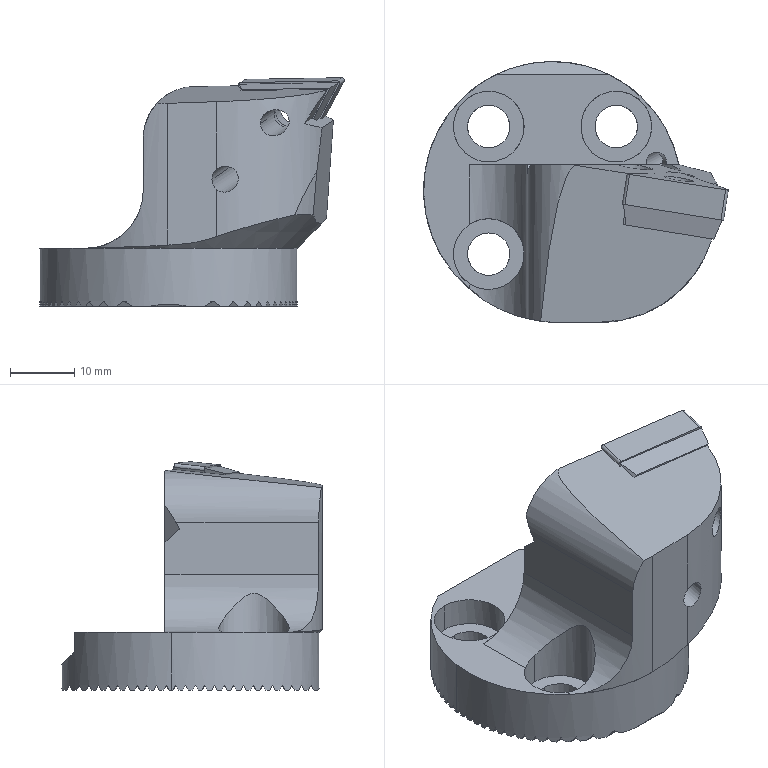NC program | Mastercam | posted with a generic post
Whole program:
%
:0001()
(MATERIAL - ALUMINUM MM - 2024)
(T7|4 FEMF |H7)
N100 G21
N102 G0 G17 G40 G80 G90 G94 G98
N104 G0 G28 G91 Z0.
N106 G0 G28 X0. Y0.
(4 FEMF |TOOL - 7|DIA. OFF. - 7|LEN. - 7|TOOL DIA. - 4.)
N108 T7 M6
N110 G0 G54 G90 X30.268 Y22.486 C8.409 B-83.617 S2500 M3
N112 G43 H7 Z44.219
N114 Z23.126
N116 Z13.126
N118 G1 Z3.126 F600.
N120 X24.704 Y19.406 Z3.065 C8.359 B-83.705 F300.
N122 Z13.065 F1200.
N124 G0 Z23.065
N126 Z44.165
N128 X24.736 Y19.424
N130 Z44.592
N132 X24.673 Y18.506
N134 C9.63 B-83.683
N136 X24.648 Y18.954
N138 Z23.453
N140 Z13.453
N142 G1 Z3.453 F600.
N144 X24.81 Y18.857 Z3.495 C9.629 B-83.682 F300.
N146 X24.972 Y18.76 Z3.496 C9.628 B-83.68
N148 X25.296 Y18.566 C9.627 B-83.678
N150 X25.944 Y18.177 Z3.497 C9.623 B-83.672
N152 X27.239 Y17.401 Z3.499 C9.617 B-83.661
N154 X29.831 Y15.847 Z3.506 C9.604 B-83.64
N156 X32.422 Y14.294 Z3.515 C9.591 B-83.618
N158 X33.718 Y13.517 Z3.52 C9.584 B-83.607
N160 X34.365 Y13.128 Z3.523 C9.581 B-83.602
N162 X34.689 Y12.934 Z3.525 C9.579 B-83.599
N164 X34.851 Y12.837 C9.578 B-83.598
N166 X34.932 Y12.789 Z3.526 B-83.597
N168 X35.013 Y12.74 Z3.483 B-83.596
N170 Z13.483 F1200.
N172 G0 Z23.483
N174 Z44.49
N176 X35.006 Y12.314
N178 M5
N180 G0 G28 G91 Z0.
N182 G0 G28 X0. Y0.
N184 G28 C0. B0.
N186 M30
%